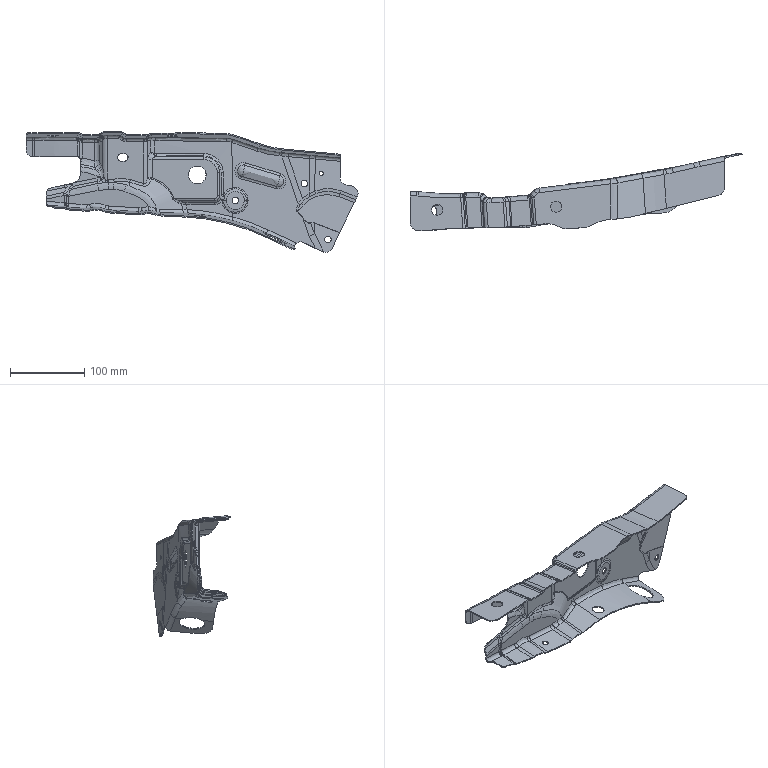Part | 1 solid | 614 faces | box 447.473 x 105.015 x 162.587 mm | volume 113532 mm3 | spline 422 | cylinder 116 | plane 43 | sphere 21 | torus 6 | other 6 | commonest cylinder face diameters 10 x29 13 x21 7 x8 20 x8 9 x6 23 x6